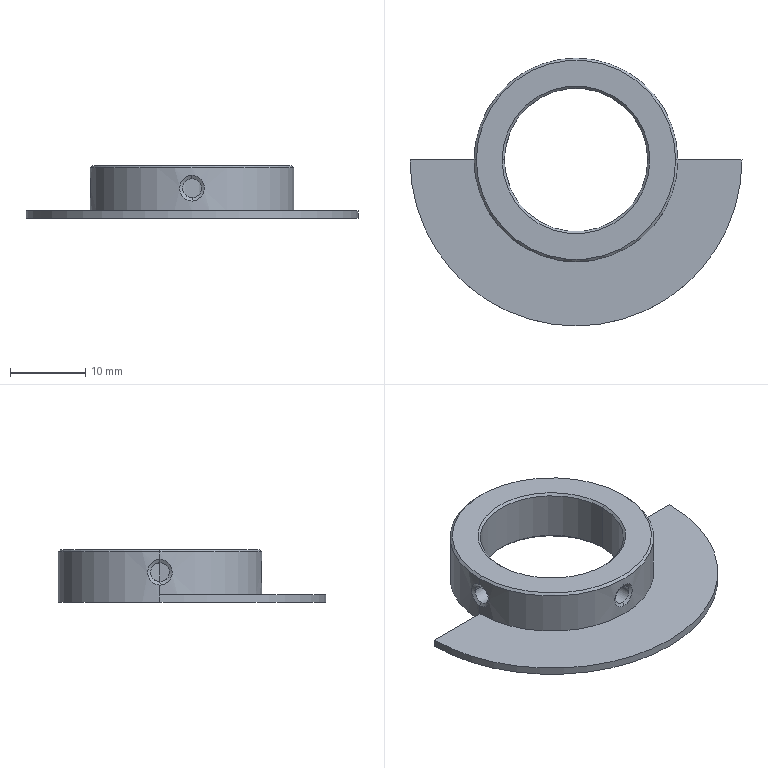Part | NX | 1 solid | 24 faces | box 44 x 35.5 x 7 mm | volume 2448 mm3 | cylinder 9 | cone 6 | plane 5 | spline 4 | commonest cylinder face diameters 2.5 x4 19 x2 27 x2 44 x1
STEP:
#1=CARTESIAN_POINT('',(13.2,0.,7.));
#2=VERTEX_POINT('',#1);
#3=CARTESIAN_POINT('',(-13.2,0.,7.));
#4=VERTEX_POINT('',#3);
#5=CARTESIAN_POINT('',(0.,0.,7.));
#6=DIRECTION('',(0.,0.,-1.));
#7=DIRECTION('',(-1.,0.,0.));
#8=AXIS2_PLACEMENT_3D('',#5,#6,#7);
#9=CIRCLE('',#8,13.2);
#10=EDGE_CURVE('',#2,#4,#9,.T.);
#11=ORIENTED_EDGE('',*,*,#10,.F.);
#12=CARTESIAN_POINT('',(0.,0.,7.));
#13=DIRECTION('',(0.,0.,-1.));
#14=DIRECTION('',(-1.,0.,0.));
#15=AXIS2_PLACEMENT_3D('',#12,#13,#14);
#16=CIRCLE('',#15,13.2);
#17=EDGE_CURVE('',#4,#2,#16,.T.);
#18=ORIENTED_EDGE('',*,*,#17,.F.);
#19=EDGE_LOOP('',(#11,#18));
#20=FACE_BOUND('',#19,.T.);
#21=CARTESIAN_POINT('',(-9.8,0.,7.));
#22=VERTEX_POINT('',#21);
#23=CARTESIAN_POINT('',(9.8,0.,7.));
#24=VERTEX_POINT('',#23);
#25=CARTESIAN_POINT('',(0.,0.,7.));
#26=DIRECTION('',(0.,0.,1.));
#27=DIRECTION('',(1.,0.,0.));
#28=AXIS2_PLACEMENT_3D('',#25,#26,#27);
#29=CIRCLE('',#28,9.8);
#30=EDGE_CURVE('',#22,#24,#29,.T.);
#31=ORIENTED_EDGE('',*,*,#30,.F.);
#32=CARTESIAN_POINT('',(0.,0.,7.));
#33=DIRECTION('',(0.,0.,1.));
#34=DIRECTION('',(1.,0.,0.));
#35=AXIS2_PLACEMENT_3D('',#32,#33,#34);
#36=CIRCLE('',#35,9.8);
#37=EDGE_CURVE('',#24,#22,#36,.T.);
#38=ORIENTED_EDGE('',*,*,#37,.F.);
#39=EDGE_LOOP('',(#31,#38));
#40=FACE_BOUND('',#39,.T.);
#41=CARTESIAN_POINT('',(0.,0.,7.));
#42=DIRECTION('',(0.,0.,1.));
#43=DIRECTION('',(1.,0.,0.));
#44=AXIS2_PLACEMENT_3D('',#41,#42,#43);
#45=PLANE('',#44);
#46=ADVANCED_FACE('',(#20,#40),#45,.T.);
#47=CARTESIAN_POINT('',(13.5,0.,0.));
#48=VERTEX_POINT('',#47);
#49=CARTESIAN_POINT('',(13.5,0.,1.));
#50=VERTEX_POINT('',#49);
#51=CARTESIAN_POINT('',(13.5,0.,0.));
#52=DIRECTION('',(0.,0.,1.));
#53=VECTOR('',#52,1000.);
#54=LINE('',#51,#53);
#55=EDGE_CURVE('',#48,#50,#54,.T.);
#56=ORIENTED_EDGE('',*,*,#55,.F.);
#57=CARTESIAN_POINT('',(-13.5,0.,0.));
#58=VERTEX_POINT('',#57);
#59=CARTESIAN_POINT('',(0.,0.,0.));
#60=DIRECTION('',(0.,0.,1.));
#61=DIRECTION('',(1.,0.,0.));
#62=AXIS2_PLACEMENT_3D('',#59,#60,#61);
#63=CIRCLE('',#62,13.5);
#64=EDGE_CURVE('',#48,#58,#63,.T.);
#65=ORIENTED_EDGE('',*,*,#64,.T.);
#66=CARTESIAN_POINT('',(-13.5,0.,1.));
#67=VERTEX_POINT('',#66);
#68=CARTESIAN_POINT('',(-13.5,0.,0.));
#69=DIRECTION('',(0.,0.,1.));
#70=VECTOR('',#69,1000.);
#71=LINE('',#68,#70);
#72=EDGE_CURVE('',#58,#67,#71,.T.);
#73=ORIENTED_EDGE('',*,*,#72,.T.);
#74=CARTESIAN_POINT('',(-13.5,0.,2.3));
#75=VERTEX_POINT('',#74);
#76=CARTESIAN_POINT('',(-13.5,0.,0.));
#77=DIRECTION('',(0.,0.,1.));
#78=VECTOR('',#77,1000.);
#79=LINE('',#76,#78);
#80=EDGE_CURVE('',#75,#67,#79,.F.);
#81=ORIENTED_EDGE('',*,*,#80,.F.);
#82=CARTESIAN_POINT('',(-13.5,0.01096,5.7));
#83=VERTEX_POINT('',#82);
#84=CARTESIAN_POINT('',(-13.5,0.,2.3));
#85=CARTESIAN_POINT('',(-13.5,0.4417,2.3));
#86=CARTESIAN_POINT('',(-13.448,1.306,2.707));
#87=CARTESIAN_POINT('',(-13.378,1.79,3.996));
#88=CARTESIAN_POINT('',(-13.447,1.313,5.283));
#89=CARTESIAN_POINT('',(-13.5,0.4559,5.697));
#90=CARTESIAN_POINT('',(-13.5,0.01096,5.7));
#91=B_SPLINE_CURVE_WITH_KNOTS('',3,(#84,#85,#86,#87,#88,#89,#90),.UNSPECIFIED.,.F.,.F.,(4,1,1,1,4),(0.,0.25,0.5,0.75,1.),.UNSPECIFIED.);
#92=EDGE_CURVE('',#83,#75,#91,.F.);
#93=ORIENTED_EDGE('',*,*,#92,.F.);
#94=CARTESIAN_POINT('',(-13.5,0.,5.7));
#95=VERTEX_POINT('',#94);
#96=CARTESIAN_POINT('',(-13.5,0.01096,5.7));
#97=CARTESIAN_POINT('',(-13.5,0.007306,5.7));
#98=CARTESIAN_POINT('',(-13.5,0.003653,5.7));
#99=CARTESIAN_POINT('',(-13.5,0.,5.7));
#100=B_SPLINE_CURVE_WITH_KNOTS('',3,(#96,#97,#98,#99),.UNSPECIFIED.,.F.,.F.,(4,4),(0.,1.),.UNSPECIFIED.);
#101=EDGE_CURVE('',#95,#83,#100,.F.);
#102=ORIENTED_EDGE('',*,*,#101,.F.);
#103=CARTESIAN_POINT('',(-13.5,0.,6.7));
#104=VERTEX_POINT('',#103);
#105=CARTESIAN_POINT('',(-13.5,0.,0.));
#106=DIRECTION('',(0.,0.,1.));
#107=VECTOR('',#106,1000.);
#108=LINE('',#105,#107);
#109=EDGE_CURVE('',#95,#104,#108,.T.);
#110=ORIENTED_EDGE('',*,*,#109,.T.);
#111=CARTESIAN_POINT('',(13.5,0.,6.7));
#112=VERTEX_POINT('',#111);
#113=CARTESIAN_POINT('',(0.,0.,6.7));
#114=DIRECTION('',(0.,0.,-1.));
#115=DIRECTION('',(-1.,0.,0.));
#116=AXIS2_PLACEMENT_3D('',#113,#114,#115);
#117=CIRCLE('',#116,13.5);
#118=EDGE_CURVE('',#104,#112,#117,.T.);
#119=ORIENTED_EDGE('',*,*,#118,.T.);
#120=CARTESIAN_POINT('',(13.5,0.,0.));
#121=DIRECTION('',(0.,0.,1.));
#122=VECTOR('',#121,1000.);
#123=LINE('',#120,#122);
#124=EDGE_CURVE('',#112,#50,#123,.F.);
#125=ORIENTED_EDGE('',*,*,#124,.T.);
#126=EDGE_LOOP('',(#56,#65,#73,#81,#93,#102,#110,#119,#125));
#127=FACE_BOUND('',#126,.T.);
#128=CARTESIAN_POINT('',(0.,0.,0.));
#129=DIRECTION('',(0.,0.,1.));
#130=DIRECTION('',(1.,0.,0.));
#131=AXIS2_PLACEMENT_3D('',#128,#129,#130);
#132=CYLINDRICAL_SURFACE('',#131,13.5);
#133=ADVANCED_FACE('',(#127),#132,.T.);
#134=CARTESIAN_POINT('',(0.009148,-13.24,2.75));
#135=VERTEX_POINT('',#134);
#136=CARTESIAN_POINT('',(1.25,-13.182,4.));
#137=VERTEX_POINT('',#136);
#138=CARTESIAN_POINT('',(0.009147,-13.24,2.75));
#139=CARTESIAN_POINT('',(0.1245,-13.24,2.751));
#140=CARTESIAN_POINT('',(0.3981,-13.236,2.779));
#141=CARTESIAN_POINT('',(0.915,-13.211,3.074));
#142=CARTESIAN_POINT('',(1.221,-13.186,3.596));
#143=CARTESIAN_POINT('',(1.25,-13.182,3.879));
#144=CARTESIAN_POINT('',(1.25,-13.182,4.));
#145=B_SPLINE_CURVE_WITH_KNOTS('',3,(#138,#139,#140,#141,#142,#143,#144),.UNSPECIFIED.,.F.,.F.,(4,1,1,1,4),(0.,0.25,0.5,0.75,1.),.UNSPECIFIED.);
#146=EDGE_CURVE('',#135,#137,#145,.T.);
#147=ORIENTED_EDGE('',*,*,#146,.F.);
#148=CARTESIAN_POINT('',(0.01305,-13.5,2.3));
#149=VERTEX_POINT('',#148);
#150=CARTESIAN_POINT('',(0.009148,-13.24,2.75));
#151=CARTESIAN_POINT('',(0.01305,-13.5,2.3));
#152=B_SPLINE_CURVE_WITH_KNOTS('',1,(#150,#151),.UNSPECIFIED.,.F.,.F.,(2,2),(0.,1.),.UNSPECIFIED.);
#153=EDGE_CURVE('',#135,#149,#152,.T.);
#154=ORIENTED_EDGE('',*,*,#153,.T.);
#155=CARTESIAN_POINT('',(-0.01314,-13.5,5.7));
#156=VERTEX_POINT('',#155);
#157=CARTESIAN_POINT('',(-0.01314,-13.5,5.7));
#158=CARTESIAN_POINT('',(0.4307,-13.5,5.704));
#159=CARTESIAN_POINT('',(1.299,-13.448,5.302));
#160=CARTESIAN_POINT('',(1.79,-13.378,4.012));
#161=CARTESIAN_POINT('',(1.317,-13.446,2.721));
#162=CARTESIAN_POINT('',(0.4589,-13.5,2.304));
#163=CARTESIAN_POINT('',(0.01305,-13.5,2.3));
#164=B_SPLINE_CURVE_WITH_KNOTS('',3,(#157,#158,#159,#160,#161,#162,#163),.UNSPECIFIED.,.F.,.F.,(4,1,1,1,4),(0.,0.25,0.5,0.75,1.),.UNSPECIFIED.);
#165=EDGE_CURVE('',#149,#156,#164,.F.);
#166=ORIENTED_EDGE('',*,*,#165,.T.);
#167=CARTESIAN_POINT('',(-0.009525,-13.24,5.25));
#168=VERTEX_POINT('',#167);
#169=CARTESIAN_POINT('',(-0.009525,-13.24,5.25));
#170=CARTESIAN_POINT('',(-0.01314,-13.5,5.7));
#171=B_SPLINE_CURVE_WITH_KNOTS('',1,(#169,#170),.UNSPECIFIED.,.F.,.F.,(2,2),(0.,1.),.UNSPECIFIED.);
#172=EDGE_CURVE('',#168,#156,#171,.T.);
#173=ORIENTED_EDGE('',*,*,#172,.F.);
#174=CARTESIAN_POINT('',(1.25,-13.182,4.));
#175=CARTESIAN_POINT('',(1.25,-13.182,4.155));
#176=CARTESIAN_POINT('',(1.178,-13.189,4.454));
#177=CARTESIAN_POINT('',(1.072,-13.198,4.655));
#178=CARTESIAN_POINT('',(0.8831,-13.212,4.907));
#179=CARTESIAN_POINT('',(0.6317,-13.225,5.086));
#180=CARTESIAN_POINT('',(0.4282,-13.234,5.187));
#181=CARTESIAN_POINT('',(0.1421,-13.24,5.251));
#182=CARTESIAN_POINT('',(-0.009525,-13.24,5.25));
#183=B_SPLINE_CURVE_WITH_KNOTS('',3,(#174,#175,#176,#177,#178,#179,#180,#181,#182),.UNSPECIFIED.,.F.,.F.,(4,1,1,1,1,1,4),(0.,0.25,0.375,0.5,0.625,0.75,1.),.UNSPECIFIED.);
#184=EDGE_CURVE('',#137,#168,#183,.T.);
#185=ORIENTED_EDGE('',*,*,#184,.F.);
#186=EDGE_LOOP('',(#147,#154,#166,#173,#185));
#187=FACE_BOUND('',#186,.T.);
#188=CARTESIAN_POINT('',(0.009148,-13.24,2.75));
#189=CARTESIAN_POINT('',(0.01305,-13.5,2.3));
#190=CARTESIAN_POINT('',(0.07196,-13.24,2.75));
#191=CARTESIAN_POINT('',(0.09975,-13.5,2.301));
#192=CARTESIAN_POINT('',(0.1349,-13.24,2.756));
#193=CARTESIAN_POINT('',(0.1865,-13.499,2.309));
#194=CARTESIAN_POINT('',(0.3998,-13.236,2.798));
#195=CARTESIAN_POINT('',(0.5485,-13.492,2.373));
#196=CARTESIAN_POINT('',(0.5907,-13.228,2.879));
#197=CARTESIAN_POINT('',(0.8061,-13.478,2.497));
#198=CARTESIAN_POINT('',(0.9215,-13.209,3.13));
#199=CARTESIAN_POINT('',(1.233,-13.445,2.855));
#200=CARTESIAN_POINT('',(1.055,-13.199,3.297));
#201=CARTESIAN_POINT('',(1.396,-13.428,3.083));
#202=CARTESIAN_POINT('',(1.227,-13.185,3.681));
#203=CARTESIAN_POINT('',(1.603,-13.405,3.591));
#204=CARTESIAN_POINT('',(1.263,-13.181,3.894));
#205=CARTESIAN_POINT('',(1.645,-13.399,3.862));
#206=CARTESIAN_POINT('',(1.228,-13.184,4.314));
#207=CARTESIAN_POINT('',(1.604,-13.404,4.406));
#208=CARTESIAN_POINT('',(1.157,-13.191,4.518));
#209=CARTESIAN_POINT('',(1.521,-13.415,4.669));
#210=CARTESIAN_POINT('',(0.925,-13.209,4.866));
#211=CARTESIAN_POINT('',(1.235,-13.444,5.14));
#212=CARTESIAN_POINT('',(0.7682,-13.219,5.007));
#213=CARTESIAN_POINT('',(1.037,-13.462,5.34));
#214=CARTESIAN_POINT('',(0.4042,-13.235,5.201));
#215=CARTESIAN_POINT('',(0.5571,-13.491,5.622));
#216=CARTESIAN_POINT('',(0.2041,-13.24,5.25));
#217=CARTESIAN_POINT('',(0.2808,-13.5,5.7));
#218=CARTESIAN_POINT('',(-0.003196,-13.24,5.25));
#219=CARTESIAN_POINT('',(-0.004398,-13.5,5.7));
#220=CARTESIAN_POINT('',(-0.006359,-13.24,5.25));
#221=CARTESIAN_POINT('',(-0.008773,-13.5,5.7));
#222=CARTESIAN_POINT('',(-0.009525,-13.24,5.25));
#223=CARTESIAN_POINT('',(-0.01314,-13.5,5.7));
#224=B_SPLINE_SURFACE_WITH_KNOTS('',3,1,((#188,#189),(#190,#191),(#192,#193),(#194,#195),(#196,#197),(#198,#199),(#200,#201),(#202,#203),(#204,#205),(#206,#207),(#208,#209),(#210,#211),(#212,#213),(#214,#215),(#216,#217),(#218,#219),(#220,#221),(#222,#223)),.RULED_SURF.,.F.,.F.,.F.,(4,2,2,2,2,2,2,2,4),(2,2),(4.613,4.839,5.568,6.302,7.029,7.759,8.489,9.216,9.227),(0.,1.),.UNSPECIFIED.);
#225=ADVANCED_FACE('',(#187),#224,.F.);
#226=CARTESIAN_POINT('',(0.,0.,1.));
#227=DIRECTION('',(0.,0.,1.));
#228=DIRECTION('',(1.,0.,0.));
#229=AXIS2_PLACEMENT_3D('',#226,#227,#228);
#230=CIRCLE('',#229,13.5);
#231=EDGE_CURVE('',#67,#50,#230,.T.);
#232=ORIENTED_EDGE('',*,*,#231,.F.);
#233=CARTESIAN_POINT('',(-22.,0.,1.));
#234=VERTEX_POINT('',#233);
#235=CARTESIAN_POINT('',(-22.,0.,1.));
#236=DIRECTION('',(1.,0.,0.));
#237=VECTOR('',#236,1000.);
#238=LINE('',#235,#237);
#239=EDGE_CURVE('',#234,#67,#238,.T.);
#240=ORIENTED_EDGE('',*,*,#239,.F.);
#241=CARTESIAN_POINT('',(22.,0.,1.));
#242=VERTEX_POINT('',#241);
#243=CARTESIAN_POINT('',(0.,0.,1.));
#244=DIRECTION('',(0.,0.,-1.));
#245=DIRECTION('',(1.,0.,0.));
#246=AXIS2_PLACEMENT_3D('',#243,#244,#245);
#247=CIRCLE('',#246,22.);
#248=EDGE_CURVE('',#242,#234,#247,.T.);
#249=ORIENTED_EDGE('',*,*,#248,.F.);
#250=CARTESIAN_POINT('',(13.5,0.,1.));
#251=DIRECTION('',(1.,0.,0.));
#252=VECTOR('',#251,1000.);
#253=LINE('',#250,#252);
#254=EDGE_CURVE('',#50,#242,#253,.T.);
#255=ORIENTED_EDGE('',*,*,#254,.F.);
#256=EDGE_LOOP('',(#232,#240,#249,#255));
#257=FACE_BOUND('',#256,.T.);
#258=CARTESIAN_POINT('',(0.,0.,1.));
#259=DIRECTION('',(0.,0.,1.));
#260=DIRECTION('',(1.,0.,0.));
#261=AXIS2_PLACEMENT_3D('',#258,#259,#260);
#262=PLANE('',#261);
#263=ADVANCED_FACE('',(#257),#262,.T.);
#264=ORIENTED_EDGE('',*,*,#55,.T.);
#265=ORIENTED_EDGE('',*,*,#254,.T.);
#266=CARTESIAN_POINT('',(22.,0.,0.));
#267=VERTEX_POINT('',#266);
#268=CARTESIAN_POINT('',(22.,0.,0.));
#269=DIRECTION('',(0.,0.,1.));
#270=VECTOR('',#269,1000.);
#271=LINE('',#268,#270);
#272=EDGE_CURVE('',#267,#242,#271,.T.);
#273=ORIENTED_EDGE('',*,*,#272,.F.);
#274=CARTESIAN_POINT('',(13.5,0.,0.));
#275=DIRECTION('',(1.,0.,0.));
#276=VECTOR('',#275,1000.);
#277=LINE('',#274,#276);
#278=EDGE_CURVE('',#48,#267,#277,.T.);
#279=ORIENTED_EDGE('',*,*,#278,.F.);
#280=EDGE_LOOP('',(#264,#265,#273,#279));
#281=FACE_BOUND('',#280,.T.);
#282=CARTESIAN_POINT('',(22.,0.,0.));
#283=DIRECTION('',(0.,1.,0.));
#284=DIRECTION('',(1.,0.,0.));
#285=AXIS2_PLACEMENT_3D('',#282,#283,#284);
#286=PLANE('',#285);
#287=ADVANCED_FACE('',(#281),#286,.T.);
#288=ORIENTED_EDGE('',*,*,#64,.F.);
#289=ORIENTED_EDGE('',*,*,#278,.T.);
#290=CARTESIAN_POINT('',(-22.,0.,0.));
#291=VERTEX_POINT('',#290);
#292=CARTESIAN_POINT('',(0.,0.,0.));
#293=DIRECTION('',(0.,0.,1.));
#294=DIRECTION('',(-1.,0.,0.));
#295=AXIS2_PLACEMENT_3D('',#292,#293,#294);
#296=CIRCLE('',#295,22.);
#297=EDGE_CURVE('',#291,#267,#296,.T.);
#298=ORIENTED_EDGE('',*,*,#297,.F.);
#299=CARTESIAN_POINT('',(-22.,0.,0.));
#300=DIRECTION('',(1.,0.,0.));
#301=VECTOR('',#300,1000.);
#302=LINE('',#299,#301);
#303=EDGE_CURVE('',#291,#58,#302,.T.);
#304=ORIENTED_EDGE('',*,*,#303,.T.);
#305=EDGE_LOOP('',(#288,#289,#298,#304));
#306=FACE_BOUND('',#305,.T.);
#307=CARTESIAN_POINT('',(-9.8,0.,0.));
#308=VERTEX_POINT('',#307);
#309=CARTESIAN_POINT('',(9.8,0.,0.));
#310=VERTEX_POINT('',#309);
#311=CARTESIAN_POINT('',(0.,0.,0.));
#312=DIRECTION('',(0.,0.,-1.));
#313=DIRECTION('',(-1.,0.,0.));
#314=AXIS2_PLACEMENT_3D('',#311,#312,#313);
#315=CIRCLE('',#314,9.8);
#316=EDGE_CURVE('',#308,#310,#315,.T.);
#317=ORIENTED_EDGE('',*,*,#316,.F.);
#318=CARTESIAN_POINT('',(0.,0.,0.));
#319=DIRECTION('',(0.,0.,-1.));
#320=DIRECTION('',(-1.,0.,0.));
#321=AXIS2_PLACEMENT_3D('',#318,#319,#320);
#322=CIRCLE('',#321,9.8);
#323=EDGE_CURVE('',#310,#308,#322,.T.);
#324=ORIENTED_EDGE('',*,*,#323,.F.);
#325=EDGE_LOOP('',(#317,#324));
#326=FACE_BOUND('',#325,.T.);
#327=CARTESIAN_POINT('',(0.,0.,0.));
#328=DIRECTION('',(0.,0.,1.));
#329=DIRECTION('',(1.,0.,0.));
#330=AXIS2_PLACEMENT_3D('',#327,#328,#329);
#331=PLANE('',#330);
#332=ADVANCED_FACE('',(#306,#326),#331,.F.);
#333=CARTESIAN_POINT('',(9.5,0.,0.3));
#334=VERTEX_POINT('',#333);
#335=CARTESIAN_POINT('',(-9.5,0.,0.3));
#336=VERTEX_POINT('',#335);
#337=CARTESIAN_POINT('',(0.,0.,0.3));
#338=DIRECTION('',(0.,0.,-1.));
#339=DIRECTION('',(-1.,0.,0.));
#340=AXIS2_PLACEMENT_3D('',#337,#338,#339);
#341=CIRCLE('',#340,9.5);
#342=EDGE_CURVE('',#334,#336,#341,.T.);
#343=ORIENTED_EDGE('',*,*,#342,.T.);
#344=CARTESIAN_POINT('',(-9.5,0.,2.75));
#345=VERTEX_POINT('',#344);
#346=CARTESIAN_POINT('',(-9.5,0.,0.));
#347=DIRECTION('',(0.,0.,1.));
#348=VECTOR('',#347,1000.);
#349=LINE('',#346,#348);
#350=EDGE_CURVE('',#336,#345,#349,.T.);
#351=ORIENTED_EDGE('',*,*,#350,.T.);
#352=CARTESIAN_POINT('',(-9.417,-1.25,4.));
#353=VERTEX_POINT('',#352);
#354=CARTESIAN_POINT('',(-9.5,0.,2.75));
#355=CARTESIAN_POINT('',(-9.5,-0.6631,2.75));
#356=CARTESIAN_POINT('',(-9.417,-1.249,3.335));
#357=CARTESIAN_POINT('',(-9.417,-1.25,4.));
#358=B_SPLINE_CURVE_WITH_KNOTS('',3,(#354,#355,#356,#357),.UNSPECIFIED.,.F.,.F.,(4,4),(0.,1.),.UNSPECIFIED.);
#359=EDGE_CURVE('',#345,#353,#358,.T.);
#360=ORIENTED_EDGE('',*,*,#359,.T.);
#361=CARTESIAN_POINT('',(-9.5,0.,5.25));
#362=VERTEX_POINT('',#361);
#363=CARTESIAN_POINT('',(-9.417,-1.25,4.));
#364=CARTESIAN_POINT('',(-9.417,-1.249,4.664));
#365=CARTESIAN_POINT('',(-9.5,-0.6634,5.25));
#366=CARTESIAN_POINT('',(-9.5,0.,5.25));
#367=B_SPLINE_CURVE_WITH_KNOTS('',3,(#363,#364,#365,#366),.UNSPECIFIED.,.F.,.F.,(4,4),(0.,1.),.UNSPECIFIED.);
#368=EDGE_CURVE('',#353,#362,#367,.T.);
#369=ORIENTED_EDGE('',*,*,#368,.T.);
#370=CARTESIAN_POINT('',(-9.5,0.,6.7));
#371=VERTEX_POINT('',#370);
#372=CARTESIAN_POINT('',(-9.5,0.,0.));
#373=DIRECTION('',(0.,0.,1.));
#374=VECTOR('',#373,1000.);
#375=LINE('',#372,#374);
#376=EDGE_CURVE('',#371,#362,#375,.F.);
#377=ORIENTED_EDGE('',*,*,#376,.F.);
#378=CARTESIAN_POINT('',(9.5,0.,6.7));
#379=VERTEX_POINT('',#378);
#380=CARTESIAN_POINT('',(0.,0.,6.7));
#381=DIRECTION('',(0.,0.,1.));
#382=DIRECTION('',(1.,0.,0.));
#383=AXIS2_PLACEMENT_3D('',#380,#381,#382);
#384=CIRCLE('',#383,9.5);
#385=EDGE_CURVE('',#371,#379,#384,.T.);
#386=ORIENTED_EDGE('',*,*,#385,.T.);
#387=CARTESIAN_POINT('',(9.5,0.,0.));
#388=DIRECTION('',(0.,0.,1.));
#389=VECTOR('',#388,1000.);
#390=LINE('',#387,#389);
#391=EDGE_CURVE('',#379,#334,#390,.F.);
#392=ORIENTED_EDGE('',*,*,#391,.T.);
#393=EDGE_LOOP('',(#343,#351,#360,#369,#377,#386,#392));
#394=FACE_BOUND('',#393,.T.);
#395=CARTESIAN_POINT('',(1.25,-9.417,4.));
#396=VERTEX_POINT('',#395);
#397=CARTESIAN_POINT('',(-1.25,-9.417,4.));
#398=VERTEX_POINT('',#397);
#399=CARTESIAN_POINT('',(-1.25,-9.417,4.));
#400=CARTESIAN_POINT('',(-1.25,-9.417,3.668));
#401=CARTESIAN_POINT('',(-0.9802,-9.459,3.024));
#402=CARTESIAN_POINT('',(0.0002555,-9.521,2.613));
#403=CARTESIAN_POINT('',(0.9792,-9.459,3.023));
#404=CARTESIAN_POINT('',(1.25,-9.417,3.668));
#405=CARTESIAN_POINT('',(1.25,-9.417,4.));
#406=B_SPLINE_CURVE_WITH_KNOTS('',3,(#399,#400,#401,#402,#403,#404,#405),.UNSPECIFIED.,.F.,.F.,(4,1,1,1,4),(0.,0.25,0.5,0.75,1.),.UNSPECIFIED.);
#407=EDGE_CURVE('',#396,#398,#406,.F.);
#408=ORIENTED_EDGE('',*,*,#407,.F.);
#409=CARTESIAN_POINT('',(1.25,-9.417,4.));
#410=CARTESIAN_POINT('',(1.25,-9.417,4.332));
#411=CARTESIAN_POINT('',(0.9799,-9.459,4.976));
#412=CARTESIAN_POINT('',(0.00004699,-9.521,5.387));
#413=CARTESIAN_POINT('',(-0.9802,-9.459,4.976));
#414=CARTESIAN_POINT('',(-1.25,-9.417,4.332));
#415=CARTESIAN_POINT('',(-1.25,-9.417,4.));
#416=B_SPLINE_CURVE_WITH_KNOTS('',3,(#409,#410,#411,#412,#413,#414,#415),.UNSPECIFIED.,.F.,.F.,(4,1,1,1,4),(0.,0.25,0.5,0.75,1.),.UNSPECIFIED.);
#417=EDGE_CURVE('',#398,#396,#416,.F.);
#418=ORIENTED_EDGE('',*,*,#417,.F.);
#419=EDGE_LOOP('',(#408,#418));
#420=FACE_BOUND('',#419,.T.);
#421=CARTESIAN_POINT('',(0.,0.,0.));
#422=DIRECTION('',(0.,0.,1.));
#423=DIRECTION('',(1.,0.,0.));
#424=AXIS2_PLACEMENT_3D('',#421,#422,#423);
#425=CYLINDRICAL_SURFACE('',#424,9.5);
#426=ADVANCED_FACE('',(#394,#420),#425,.F.);
#427=ORIENTED_EDGE('',*,*,#72,.F.);
#428=ORIENTED_EDGE('',*,*,#303,.F.);
#429=CARTESIAN_POINT('',(-22.,0.,0.));
#430=DIRECTION('',(0.,0.,1.));
#431=VECTOR('',#430,1000.);
#432=LINE('',#429,#431);
#433=EDGE_CURVE('',#291,#234,#432,.T.);
#434=ORIENTED_EDGE('',*,*,#433,.T.);
#435=ORIENTED_EDGE('',*,*,#239,.T.);
#436=EDGE_LOOP('',(#427,#428,#434,#435));
#437=FACE_BOUND('',#436,.T.);
#438=CARTESIAN_POINT('',(-13.5,0.,0.));
#439=DIRECTION('',(0.,1.,0.));
#440=DIRECTION('',(1.,0.,0.));
#441=AXIS2_PLACEMENT_3D('',#438,#439,#440);
#442=PLANE('',#441);
#443=ADVANCED_FACE('',(#437),#442,.T.);
#444=ORIENTED_EDGE('',*,*,#297,.T.);
#445=ORIENTED_EDGE('',*,*,#272,.T.);
#446=ORIENTED_EDGE('',*,*,#248,.T.);
#447=ORIENTED_EDGE('',*,*,#433,.F.);
#448=EDGE_LOOP('',(#444,#445,#446,#447));
#449=FACE_BOUND('',#448,.T.);
#450=CARTESIAN_POINT('',(0.,0.,0.));
#451=DIRECTION('',(0.,0.,1.));
#452=DIRECTION('',(1.,0.,0.));
#453=AXIS2_PLACEMENT_3D('',#450,#451,#452);
#454=CYLINDRICAL_SURFACE('',#453,22.);
#455=ADVANCED_FACE('',(#449),#454,.T.);
#456=ORIENTED_EDGE('',*,*,#407,.T.);
#457=CARTESIAN_POINT('',(-1.25,-13.182,4.));
#458=VERTEX_POINT('',#457);
#459=CARTESIAN_POINT('',(-1.25,-13.5,4.));
#460=DIRECTION('',(0.,-1.,0.));
#461=VECTOR('',#460,1000.);
#462=LINE('',#459,#461);
#463=EDGE_CURVE('',#458,#398,#462,.F.);
#464=ORIENTED_EDGE('',*,*,#463,.F.);
#465=CARTESIAN_POINT('',(-1.25,-13.182,4.));
#466=CARTESIAN_POINT('',(-1.25,-13.182,3.841));
#467=CARTESIAN_POINT('',(-1.178,-13.189,3.547));
#468=CARTESIAN_POINT('',(-1.072,-13.198,3.344));
#469=CARTESIAN_POINT('',(-0.8826,-13.212,3.093));
#470=CARTESIAN_POINT('',(-0.6331,-13.225,2.915));
#471=CARTESIAN_POINT('',(-0.4278,-13.234,2.813));
#472=CARTESIAN_POINT('',(-0.1458,-13.24,2.749));
#473=CARTESIAN_POINT('',(0.009147,-13.24,2.75));
#474=B_SPLINE_CURVE_WITH_KNOTS('',3,(#465,#466,#467,#468,#469,#470,#471,#472,#473),.UNSPECIFIED.,.F.,.F.,(4,1,1,1,1,1,4),(0.,0.25,0.375,0.5,0.625,0.75,1.),.UNSPECIFIED.);
#475=EDGE_CURVE('',#458,#135,#474,.T.);
#476=ORIENTED_EDGE('',*,*,#475,.T.);
#477=ORIENTED_EDGE('',*,*,#146,.T.);
#478=CARTESIAN_POINT('',(1.25,-13.5,4.));
#479=DIRECTION('',(0.,-1.,0.));
#480=VECTOR('',#479,1000.);
#481=LINE('',#478,#480);
#482=EDGE_CURVE('',#137,#396,#481,.F.);
#483=ORIENTED_EDGE('',*,*,#482,.T.);
#484=EDGE_LOOP('',(#456,#464,#476,#477,#483));
#485=FACE_BOUND('',#484,.T.);
#486=CARTESIAN_POINT('',(0.,-13.5,4.));
#487=DIRECTION('',(0.,-1.,0.));
#488=DIRECTION('',(-1.,0.,0.));
#489=AXIS2_PLACEMENT_3D('',#486,#487,#488);
#490=CYLINDRICAL_SURFACE('',#489,1.25);
#491=ADVANCED_FACE('',(#485),#490,.F.);
#492=ORIENTED_EDGE('',*,*,#368,.F.);
#493=CARTESIAN_POINT('',(-13.182,-1.25,4.));
#494=VERTEX_POINT('',#493);
#495=CARTESIAN_POINT('',(-13.5,-1.25,4.));
#496=DIRECTION('',(-1.,0.,0.));
#497=VECTOR('',#496,1000.);
#498=LINE('',#495,#497);
#499=EDGE_CURVE('',#353,#494,#498,.T.);
#500=ORIENTED_EDGE('',*,*,#499,.T.);
#501=CARTESIAN_POINT('',(-13.24,0.007631,5.25));
#502=VERTEX_POINT('',#501);
#503=CARTESIAN_POINT('',(-13.182,-1.25,4.));
#504=CARTESIAN_POINT('',(-13.182,-1.25,4.159));
#505=CARTESIAN_POINT('',(-13.189,-1.179,4.452));
#506=CARTESIAN_POINT('',(-13.198,-1.072,4.656));
#507=CARTESIAN_POINT('',(-13.212,-0.8832,4.907));
#508=CARTESIAN_POINT('',(-13.225,-0.6338,5.085));
#509=CARTESIAN_POINT('',(-13.234,-0.429,5.187));
#510=CARTESIAN_POINT('',(-13.24,-0.1471,5.251));
#511=CARTESIAN_POINT('',(-13.24,0.00763,5.25));
#512=B_SPLINE_CURVE_WITH_KNOTS('',3,(#503,#504,#505,#506,#507,#508,#509,#510,#511),.UNSPECIFIED.,.F.,.F.,(4,1,1,1,1,1,4),(0.,0.25,0.375,0.5,0.625,0.75,1.),.UNSPECIFIED.);
#513=EDGE_CURVE('',#494,#502,#512,.T.);
#514=ORIENTED_EDGE('',*,*,#513,.T.);
#515=CARTESIAN_POINT('',(-13.182,1.25,4.));
#516=VERTEX_POINT('',#515);
#517=CARTESIAN_POINT('',(-13.24,0.00763,5.25));
#518=CARTESIAN_POINT('',(-13.24,0.1583,5.249));
#519=CARTESIAN_POINT('',(-13.234,0.4417,5.182));
#520=CARTESIAN_POINT('',(-13.225,0.6422,5.08));
#521=CARTESIAN_POINT('',(-13.211,0.8894,4.9));
#522=CARTESIAN_POINT('',(-13.197,1.076,4.649));
#523=CARTESIAN_POINT('',(-13.188,1.179,4.449));
#524=CARTESIAN_POINT('',(-13.182,1.25,4.158));
#525=CARTESIAN_POINT('',(-13.182,1.25,4.));
#526=B_SPLINE_CURVE_WITH_KNOTS('',3,(#517,#518,#519,#520,#521,#522,#523,#524,#525),.UNSPECIFIED.,.F.,.F.,(4,1,1,1,1,1,4),(0.,0.25,0.375,0.5,0.625,0.75,1.),.UNSPECIFIED.);
#527=EDGE_CURVE('',#502,#516,#526,.T.);
#528=ORIENTED_EDGE('',*,*,#527,.T.);
#529=CARTESIAN_POINT('',(-9.417,1.25,4.));
#530=VERTEX_POINT('',#529);
#531=CARTESIAN_POINT('',(-13.5,1.25,4.));
#532=DIRECTION('',(-1.,0.,0.));
#533=VECTOR('',#532,1000.);
#534=LINE('',#531,#533);
#535=EDGE_CURVE('',#530,#516,#534,.T.);
#536=ORIENTED_EDGE('',*,*,#535,.F.);
#537=CARTESIAN_POINT('',(-9.417,1.25,4.));
#538=CARTESIAN_POINT('',(-9.417,1.25,4.155));
#539=CARTESIAN_POINT('',(-9.426,1.181,4.444));
#540=CARTESIAN_POINT('',(-9.439,1.079,4.645));
#541=CARTESIAN_POINT('',(-9.459,0.8946,4.895));
#542=CARTESIAN_POINT('',(-9.478,0.6462,5.077));
#543=CARTESIAN_POINT('',(-9.491,0.4429,5.182));
#544=CARTESIAN_POINT('',(-9.5,0.1549,5.25));
#545=CARTESIAN_POINT('',(-9.5,0.,5.25));
#546=B_SPLINE_CURVE_WITH_KNOTS('',3,(#537,#538,#539,#540,#541,#542,#543,#544,#545),.UNSPECIFIED.,.F.,.F.,(4,1,1,1,1,1,4),(0.,0.25,0.375,0.5,0.625,0.75,1.),.UNSPECIFIED.);
#547=EDGE_CURVE('',#362,#530,#546,.F.);
#548=ORIENTED_EDGE('',*,*,#547,.F.);
#549=EDGE_LOOP('',(#492,#500,#514,#528,#536,#548));
#550=FACE_BOUND('',#549,.T.);
#551=CARTESIAN_POINT('',(-13.5,0.,4.));
#552=DIRECTION('',(-1.,0.,0.));
#553=DIRECTION('',(0.,1.,0.));
#554=AXIS2_PLACEMENT_3D('',#551,#552,#553);
#555=CYLINDRICAL_SURFACE('',#554,1.25);
#556=ADVANCED_FACE('',(#550),#555,.F.);
#557=ORIENTED_EDGE('',*,*,#513,.F.);
#558=CARTESIAN_POINT('',(-13.24,-0.008007,2.75));
#559=VERTEX_POINT('',#558);
#560=CARTESIAN_POINT('',(-13.24,-0.008007,2.75));
#561=CARTESIAN_POINT('',(-13.24,-0.1601,2.751));
#562=CARTESIAN_POINT('',(-13.234,-0.4439,2.819));
#563=CARTESIAN_POINT('',(-13.225,-0.6419,2.92));
#564=CARTESIAN_POINT('',(-13.211,-0.8903,3.101));
#565=CARTESIAN_POINT('',(-13.198,-1.073,3.347));
#566=CARTESIAN_POINT('',(-13.188,-1.181,3.553));
#567=CARTESIAN_POINT('',(-13.182,-1.25,3.842));
#568=CARTESIAN_POINT('',(-13.182,-1.25,4.));
#569=B_SPLINE_CURVE_WITH_KNOTS('',3,(#560,#561,#562,#563,#564,#565,#566,#567,#568),.UNSPECIFIED.,.F.,.F.,(4,1,1,1,1,1,4),(0.,0.25,0.375,0.5,0.625,0.75,1.),.UNSPECIFIED.);
#570=EDGE_CURVE('',#559,#494,#569,.T.);
#571=ORIENTED_EDGE('',*,*,#570,.F.);
#572=CARTESIAN_POINT('',(-13.5,-0.01105,2.3));
#573=VERTEX_POINT('',#572);
#574=CARTESIAN_POINT('',(-13.24,-0.008007,2.75));
#575=CARTESIAN_POINT('',(-13.5,-0.01105,2.3));
#576=B_SPLINE_CURVE_WITH_KNOTS('',1,(#574,#575),.UNSPECIFIED.,.F.,.F.,(2,2),(0.,1.),.UNSPECIFIED.);
#577=EDGE_CURVE('',#559,#573,#576,.T.);
#578=ORIENTED_EDGE('',*,*,#577,.T.);
#579=CARTESIAN_POINT('',(-13.5,0.,5.7));
#580=CARTESIAN_POINT('',(-13.5,-0.4479,5.699));
#581=CARTESIAN_POINT('',(-13.448,-1.303,5.293));
#582=CARTESIAN_POINT('',(-13.378,-1.79,4.006));
#583=CARTESIAN_POINT('',(-13.446,-1.314,2.718));
#584=CARTESIAN_POINT('',(-13.5,-0.4559,2.303));
#585=CARTESIAN_POINT('',(-13.5,-0.01105,2.3));
#586=B_SPLINE_CURVE_WITH_KNOTS('',3,(#579,#580,#581,#582,#583,#584,#585),.UNSPECIFIED.,.F.,.F.,(4,1,1,1,4),(0.,0.25,0.5,0.75,1.),.UNSPECIFIED.);
#587=EDGE_CURVE('',#573,#95,#586,.F.);
#588=ORIENTED_EDGE('',*,*,#587,.T.);
#589=ORIENTED_EDGE('',*,*,#101,.T.);
#590=CARTESIAN_POINT('',(-13.24,0.007631,5.25));
#591=CARTESIAN_POINT('',(-13.5,0.01096,5.7));
#592=B_SPLINE_CURVE_WITH_KNOTS('',1,(#590,#591),.UNSPECIFIED.,.F.,.F.,(2,2),(0.,1.),.UNSPECIFIED.);
#593=EDGE_CURVE('',#502,#83,#592,.T.);
#594=ORIENTED_EDGE('',*,*,#593,.F.);
#595=EDGE_LOOP('',(#557,#571,#578,#588,#589,#594));
#596=FACE_BOUND('',#595,.T.);
#597=CARTESIAN_POINT('',(-13.24,-0.008007,2.75));
#598=CARTESIAN_POINT('',(-13.5,-0.01105,2.3));
#599=CARTESIAN_POINT('',(-13.24,-0.01372,2.75));
#600=CARTESIAN_POINT('',(-13.5,-0.01893,2.3));
#601=CARTESIAN_POINT('',(-13.24,-0.01944,2.75));
#602=CARTESIAN_POINT('',(-13.5,-0.02682,2.3));
#603=CARTESIAN_POINT('',(-13.24,-0.04897,2.751));
#604=CARTESIAN_POINT('',(-13.5,-0.06756,2.301));
#605=CARTESIAN_POINT('',(-13.24,-0.07275,2.752));
#606=CARTESIAN_POINT('',(-13.5,-0.1004,2.303));
#607=CARTESIAN_POINT('',(-13.239,-0.1958,2.761));
#608=CARTESIAN_POINT('',(-13.498,-0.2697,2.318));
#609=CARTESIAN_POINT('',(-13.237,-0.2935,2.781));
#610=CARTESIAN_POINT('',(-13.495,-0.4045,2.348));
#611=CARTESIAN_POINT('',(-13.229,-0.5846,2.876));
#612=CARTESIAN_POINT('',(-13.479,-0.7967,2.49));
#613=CARTESIAN_POINT('',(-13.219,-0.7622,2.987));
#614=CARTESIAN_POINT('',(-13.462,-1.029,2.655));
#615=CARTESIAN_POINT('',(-13.2,-1.049,3.289));
#616=CARTESIAN_POINT('',(-13.429,-1.39,3.073));
#617=CARTESIAN_POINT('',(-13.191,-1.154,3.475));
#618=CARTESIAN_POINT('',(-13.415,-1.515,3.319));
#619=CARTESIAN_POINT('',(-13.181,-1.262,3.881));
#620=CARTESIAN_POINT('',(-13.4,-1.644,3.849));
#621=CARTESIAN_POINT('',(-13.181,-1.264,4.097));
#622=CARTESIAN_POINT('',(-13.399,-1.646,4.123));
#623=CARTESIAN_POINT('',(-13.19,-1.162,4.507));
#624=CARTESIAN_POINT('',(-13.414,-1.525,4.657));
#625=CARTESIAN_POINT('',(-13.199,-1.059,4.697));
#626=CARTESIAN_POINT('',(-13.428,-1.402,4.908));
#627=CARTESIAN_POINT('',(-13.218,-0.7742,5.003));
#628=CARTESIAN_POINT('',(-13.461,-1.045,5.332));
#629=CARTESIAN_POINT('',(-13.228,-0.598,5.117));
#630=CARTESIAN_POINT('',(-13.478,-0.8148,5.499));
#631=CARTESIAN_POINT('',(-13.238,-0.2698,5.229));
#632=CARTESIAN_POINT('',(-13.496,-0.3728,5.667));
#633=CARTESIAN_POINT('',(-13.24,-0.1314,5.251));
#634=CARTESIAN_POINT('',(-13.5,-0.181,5.701));
#635=CARTESIAN_POINT('',(-13.24,0.007631,5.25));
#636=CARTESIAN_POINT('',(-13.5,0.01096,5.7));
#637=B_SPLINE_SURFACE_WITH_KNOTS('',3,1,((#597,#598),(#599,#600),(#601,#602),(#603,#604),(#605,#606),(#607,#608),(#609,#610),(#611,#612),(#613,#614),(#615,#616),(#617,#618),(#619,#620),(#621,#622),(#623,#624),(#625,#626),(#627,#628),(#629,#630),(#631,#632),(#633,#634),(#635,#636)),.RULED_SURF.,.F.,.F.,.F.,(4,2,2,2,2,2,2,2,2,4),(2,2),(0.,0.02041,0.1054,0.4605,1.193,1.92,2.648,3.383,4.114,4.613),(0.,1.),.UNSPECIFIED.);
#638=ADVANCED_FACE('',(#596),#637,.F.);
#639=CARTESIAN_POINT('',(0.,0.,6.7));
#640=DIRECTION('',(0.,0.,-1.));
#641=DIRECTION('',(-1.,0.,0.));
#642=AXIS2_PLACEMENT_3D('',#639,#640,#641);
#643=CIRCLE('',#642,13.5);
#644=EDGE_CURVE('',#112,#104,#643,.T.);
#645=ORIENTED_EDGE('',*,*,#644,.F.);
#646=CARTESIAN_POINT('',(13.5,0.,6.7));
#647=DIRECTION('',(0.7071,0.,-0.7071));
#648=VECTOR('',#647,1000.);
#649=LINE('',#646,#648);
#650=EDGE_CURVE('',#112,#2,#649,.F.);
#651=ORIENTED_EDGE('',*,*,#650,.T.);
#652=ORIENTED_EDGE('',*,*,#10,.T.);
#653=CARTESIAN_POINT('',(-13.5,0.,6.7));
#654=DIRECTION('',(-0.7071,0.,-0.7071));
#655=VECTOR('',#654,1000.);
#656=LINE('',#653,#655);
#657=EDGE_CURVE('',#104,#4,#656,.F.);
#658=ORIENTED_EDGE('',*,*,#657,.F.);
#659=EDGE_LOOP('',(#645,#651,#652,#658));
#660=FACE_BOUND('',#659,.T.);
#661=CARTESIAN_POINT('',(0.,0.,6.7));
#662=DIRECTION('',(0.,0.,-1.));
#663=DIRECTION('',(-1.,0.,0.));
#664=AXIS2_PLACEMENT_3D('',#661,#662,#663);
#665=CONICAL_SURFACE('',#664,13.5,0.7854);
#666=ADVANCED_FACE('',(#660),#665,.T.);
#667=ORIENTED_EDGE('',*,*,#30,.T.);
#668=CARTESIAN_POINT('',(9.8,0.,7.));
#669=DIRECTION('',(0.7071,0.,0.7071));
#670=VECTOR('',#669,1000.);
#671=LINE('',#668,#670);
#672=EDGE_CURVE('',#379,#24,#671,.T.);
#673=ORIENTED_EDGE('',*,*,#672,.F.);
#674=ORIENTED_EDGE('',*,*,#385,.F.);
#675=CARTESIAN_POINT('',(-9.8,0.,7.));
#676=DIRECTION('',(-0.7071,0.,0.7071));
#677=VECTOR('',#676,1000.);
#678=LINE('',#675,#677);
#679=EDGE_CURVE('',#371,#22,#678,.T.);
#680=ORIENTED_EDGE('',*,*,#679,.T.);
#681=EDGE_LOOP('',(#667,#673,#674,#680));
#682=FACE_BOUND('',#681,.T.);
#683=CARTESIAN_POINT('',(0.,0.,7.));
#684=DIRECTION('',(0.,0.,1.));
#685=DIRECTION('',(1.,0.,0.));
#686=AXIS2_PLACEMENT_3D('',#683,#684,#685);
#687=CONICAL_SURFACE('',#686,9.8,0.7854);
#688=ADVANCED_FACE('',(#682),#687,.F.);
#689=ORIENTED_EDGE('',*,*,#342,.F.);
#690=CARTESIAN_POINT('',(9.8,0.,0.));
#691=DIRECTION('',(0.7071,0.,-0.7071));
#692=VECTOR('',#691,1000.);
#693=LINE('',#690,#692);
#694=EDGE_CURVE('',#334,#310,#693,.T.);
#695=ORIENTED_EDGE('',*,*,#694,.T.);
#696=ORIENTED_EDGE('',*,*,#323,.T.);
#697=CARTESIAN_POINT('',(-9.8,0.,0.));
#698=DIRECTION('',(-0.7071,0.,-0.7071));
#699=VECTOR('',#698,1000.);
#700=LINE('',#697,#699);
#701=EDGE_CURVE('',#336,#308,#700,.T.);
#702=ORIENTED_EDGE('',*,*,#701,.F.);
#703=EDGE_LOOP('',(#689,#695,#696,#702));
#704=FACE_BOUND('',#703,.T.);
#705=CARTESIAN_POINT('',(0.,0.,0.));
#706=DIRECTION('',(0.,0.,-1.));
#707=DIRECTION('',(-1.,0.,0.));
#708=AXIS2_PLACEMENT_3D('',#705,#706,#707);
#709=CONICAL_SURFACE('',#708,9.8,0.7854);
#710=ADVANCED_FACE('',(#704),#709,.F.);
#711=ORIENTED_EDGE('',*,*,#657,.T.);
#712=ORIENTED_EDGE('',*,*,#17,.T.);
#713=ORIENTED_EDGE('',*,*,#650,.F.);
#714=ORIENTED_EDGE('',*,*,#118,.F.);
#715=EDGE_LOOP('',(#711,#712,#713,#714));
#716=FACE_BOUND('',#715,.T.);
#717=CARTESIAN_POINT('',(0.,0.,6.7));
#718=DIRECTION('',(0.,0.,-1.));
#719=DIRECTION('',(-1.,0.,0.));
#720=AXIS2_PLACEMENT_3D('',#717,#718,#719);
#721=CONICAL_SURFACE('',#720,13.5,0.7854);
#722=ADVANCED_FACE('',(#716),#721,.T.);
#723=ORIENTED_EDGE('',*,*,#535,.T.);
#724=CARTESIAN_POINT('',(-13.182,1.25,4.));
#725=CARTESIAN_POINT('',(-13.182,1.25,3.845));
#726=CARTESIAN_POINT('',(-13.189,1.179,3.547));
#727=CARTESIAN_POINT('',(-13.198,1.072,3.345));
#728=CARTESIAN_POINT('',(-13.212,0.8837,3.094));
#729=CARTESIAN_POINT('',(-13.225,0.6324,2.914));
#730=CARTESIAN_POINT('',(-13.234,0.4295,2.813));
#731=CARTESIAN_POINT('',(-13.24,0.1435,2.749));
#732=CARTESIAN_POINT('',(-13.24,-0.008007,2.75));
#733=B_SPLINE_CURVE_WITH_KNOTS('',3,(#724,#725,#726,#727,#728,#729,#730,#731,#732),.UNSPECIFIED.,.F.,.F.,(4,1,1,1,1,1,4),(0.,0.25,0.375,0.5,0.625,0.75,1.),.UNSPECIFIED.);
#734=EDGE_CURVE('',#516,#559,#733,.T.);
#735=ORIENTED_EDGE('',*,*,#734,.T.);
#736=ORIENTED_EDGE('',*,*,#570,.T.);
#737=ORIENTED_EDGE('',*,*,#499,.F.);
#738=ORIENTED_EDGE('',*,*,#359,.F.);
#739=CARTESIAN_POINT('',(-9.5,0.,2.75));
#740=CARTESIAN_POINT('',(-9.5,0.1548,2.75));
#741=CARTESIAN_POINT('',(-9.491,0.443,2.818));
#742=CARTESIAN_POINT('',(-9.478,0.6461,2.922));
#743=CARTESIAN_POINT('',(-9.459,0.8947,3.105));
#744=CARTESIAN_POINT('',(-9.439,1.079,3.356));
#745=CARTESIAN_POINT('',(-9.426,1.181,3.556));
#746=CARTESIAN_POINT('',(-9.417,1.25,3.845));
#747=CARTESIAN_POINT('',(-9.417,1.25,4.));
#748=B_SPLINE_CURVE_WITH_KNOTS('',3,(#739,#740,#741,#742,#743,#744,#745,#746,#747),.UNSPECIFIED.,.F.,.F.,(4,1,1,1,1,1,4),(0.,0.25,0.375,0.5,0.625,0.75,1.),.UNSPECIFIED.);
#749=EDGE_CURVE('',#530,#345,#748,.F.);
#750=ORIENTED_EDGE('',*,*,#749,.F.);
#751=EDGE_LOOP('',(#723,#735,#736,#737,#738,#750));
#752=FACE_BOUND('',#751,.T.);
#753=CARTESIAN_POINT('',(-13.5,0.,4.));
#754=DIRECTION('',(-1.,0.,0.));
#755=DIRECTION('',(0.,1.,0.));
#756=AXIS2_PLACEMENT_3D('',#753,#754,#755);
#757=CYLINDRICAL_SURFACE('',#756,1.25);
#758=ADVANCED_FACE('',(#752),#757,.F.);
#759=ORIENTED_EDGE('',*,*,#644,.T.);
#760=ORIENTED_EDGE('',*,*,#109,.F.);
#761=ORIENTED_EDGE('',*,*,#587,.F.);
#762=CARTESIAN_POINT('',(-13.5,0.,2.3));
#763=CARTESIAN_POINT('',(-13.5,-0.003678,2.3));
#764=CARTESIAN_POINT('',(-13.5,-0.007364,2.3));
#765=CARTESIAN_POINT('',(-13.5,-0.01105,2.3));
#766=B_SPLINE_CURVE_WITH_KNOTS('',3,(#762,#763,#764,#765),.UNSPECIFIED.,.F.,.F.,(4,4),(9.217,9.227),.UNSPECIFIED.);
#767=EDGE_CURVE('',#75,#573,#766,.T.);
#768=ORIENTED_EDGE('',*,*,#767,.F.);
#769=ORIENTED_EDGE('',*,*,#80,.T.);
#770=ORIENTED_EDGE('',*,*,#231,.T.);
#771=ORIENTED_EDGE('',*,*,#124,.F.);
#772=EDGE_LOOP('',(#759,#760,#761,#768,#769,#770,#771));
#773=FACE_BOUND('',#772,.T.);
#774=ORIENTED_EDGE('',*,*,#165,.F.);
#775=CARTESIAN_POINT('',(0.01305,-13.5,2.3));
#776=CARTESIAN_POINT('',(-0.4359,-13.5,2.297));
#777=CARTESIAN_POINT('',(-1.296,-13.449,2.698));
#778=CARTESIAN_POINT('',(-1.791,-13.378,3.986));
#779=CARTESIAN_POINT('',(-1.318,-13.446,5.278));
#780=CARTESIAN_POINT('',(-0.4589,-13.5,5.696));
#781=CARTESIAN_POINT('',(-0.01314,-13.5,5.7));
#782=B_SPLINE_CURVE_WITH_KNOTS('',3,(#775,#776,#777,#778,#779,#780,#781),.UNSPECIFIED.,.F.,.F.,(4,1,1,1,4),(0.,0.25,0.5,0.75,1.),.UNSPECIFIED.);
#783=EDGE_CURVE('',#156,#149,#782,.F.);
#784=ORIENTED_EDGE('',*,*,#783,.F.);
#785=EDGE_LOOP('',(#774,#784));
#786=FACE_BOUND('',#785,.T.);
#787=CARTESIAN_POINT('',(0.,0.,0.));
#788=DIRECTION('',(0.,0.,1.));
#789=DIRECTION('',(1.,0.,0.));
#790=AXIS2_PLACEMENT_3D('',#787,#788,#789);
#791=CYLINDRICAL_SURFACE('',#790,13.5);
#792=ADVANCED_FACE('',(#773,#786),#791,.T.);
#793=ORIENTED_EDGE('',*,*,#350,.F.);
#794=CARTESIAN_POINT('',(0.,0.,0.3));
#795=DIRECTION('',(0.,0.,-1.));
#796=DIRECTION('',(-1.,0.,0.));
#797=AXIS2_PLACEMENT_3D('',#794,#795,#796);
#798=CIRCLE('',#797,9.5);
#799=EDGE_CURVE('',#336,#334,#798,.T.);
#800=ORIENTED_EDGE('',*,*,#799,.T.);
#801=ORIENTED_EDGE('',*,*,#391,.F.);
#802=CARTESIAN_POINT('',(0.,0.,6.7));
#803=DIRECTION('',(0.,0.,1.));
#804=DIRECTION('',(1.,0.,0.));
#805=AXIS2_PLACEMENT_3D('',#802,#803,#804);
#806=CIRCLE('',#805,9.5);
#807=EDGE_CURVE('',#379,#371,#806,.T.);
#808=ORIENTED_EDGE('',*,*,#807,.T.);
#809=ORIENTED_EDGE('',*,*,#376,.T.);
#810=ORIENTED_EDGE('',*,*,#547,.T.);
#811=ORIENTED_EDGE('',*,*,#749,.T.);
#812=EDGE_LOOP('',(#793,#800,#801,#808,#809,#810,#811));
#813=FACE_BOUND('',#812,.T.);
#814=CARTESIAN_POINT('',(0.,0.,0.));
#815=DIRECTION('',(0.,0.,1.));
#816=DIRECTION('',(1.,0.,0.));
#817=AXIS2_PLACEMENT_3D('',#814,#815,#816);
#818=CYLINDRICAL_SURFACE('',#817,9.5);
#819=ADVANCED_FACE('',(#813),#818,.F.);
#820=ORIENTED_EDGE('',*,*,#672,.T.);
#821=ORIENTED_EDGE('',*,*,#37,.T.);
#822=ORIENTED_EDGE('',*,*,#679,.F.);
#823=ORIENTED_EDGE('',*,*,#807,.F.);
#824=EDGE_LOOP('',(#820,#821,#822,#823));
#825=FACE_BOUND('',#824,.T.);
#826=CARTESIAN_POINT('',(0.,0.,7.));
#827=DIRECTION('',(0.,0.,1.));
#828=DIRECTION('',(1.,0.,0.));
#829=AXIS2_PLACEMENT_3D('',#826,#827,#828);
#830=CONICAL_SURFACE('',#829,9.8,0.7854);
#831=ADVANCED_FACE('',(#825),#830,.F.);
#832=ORIENTED_EDGE('',*,*,#463,.T.);
#833=ORIENTED_EDGE('',*,*,#417,.T.);
#834=ORIENTED_EDGE('',*,*,#482,.F.);
#835=ORIENTED_EDGE('',*,*,#184,.T.);
#836=CARTESIAN_POINT('',(-0.009525,-13.24,5.25));
#837=CARTESIAN_POINT('',(-0.1614,-13.24,5.249));
#838=CARTESIAN_POINT('',(-0.4452,-13.234,5.18));
#839=CARTESIAN_POINT('',(-0.6425,-13.225,5.08));
#840=CARTESIAN_POINT('',(-0.891,-13.211,4.899));
#841=CARTESIAN_POINT('',(-1.074,-13.198,4.653));
#842=CARTESIAN_POINT('',(-1.181,-13.188,4.446));
#843=CARTESIAN_POINT('',(-1.25,-13.182,4.158));
#844=CARTESIAN_POINT('',(-1.25,-13.182,4.));
#845=B_SPLINE_CURVE_WITH_KNOTS('',3,(#836,#837,#838,#839,#840,#841,#842,#843,#844),.UNSPECIFIED.,.F.,.F.,(4,1,1,1,1,1,4),(0.,0.25,0.375,0.5,0.625,0.75,1.),.UNSPECIFIED.);
#846=EDGE_CURVE('',#168,#458,#845,.T.);
#847=ORIENTED_EDGE('',*,*,#846,.T.);
#848=EDGE_LOOP('',(#832,#833,#834,#835,#847));
#849=FACE_BOUND('',#848,.T.);
#850=CARTESIAN_POINT('',(0.,-13.5,4.));
#851=DIRECTION('',(0.,-1.,0.));
#852=DIRECTION('',(-1.,0.,0.));
#853=AXIS2_PLACEMENT_3D('',#850,#851,#852);
#854=CYLINDRICAL_SURFACE('',#853,1.25);
#855=ADVANCED_FACE('',(#849),#854,.F.);
#856=ORIENTED_EDGE('',*,*,#316,.T.);
#857=ORIENTED_EDGE('',*,*,#694,.F.);
#858=ORIENTED_EDGE('',*,*,#799,.F.);
#859=ORIENTED_EDGE('',*,*,#701,.T.);
#860=EDGE_LOOP('',(#856,#857,#858,#859));
#861=FACE_BOUND('',#860,.T.);
#862=CARTESIAN_POINT('',(0.,0.,0.));
#863=DIRECTION('',(0.,0.,-1.));
#864=DIRECTION('',(-1.,0.,0.));
#865=AXIS2_PLACEMENT_3D('',#862,#863,#864);
#866=CONICAL_SURFACE('',#865,9.8,0.7854);
#867=ADVANCED_FACE('',(#861),#866,.F.);
#868=ORIENTED_EDGE('',*,*,#593,.T.);
#869=ORIENTED_EDGE('',*,*,#92,.T.);
#870=ORIENTED_EDGE('',*,*,#767,.T.);
#871=ORIENTED_EDGE('',*,*,#577,.F.);
#872=ORIENTED_EDGE('',*,*,#734,.F.);
#873=ORIENTED_EDGE('',*,*,#527,.F.);
#874=EDGE_LOOP('',(#868,#869,#870,#871,#872,#873));
#875=FACE_BOUND('',#874,.T.);
#876=CARTESIAN_POINT('',(-13.24,0.007631,5.25));
#877=CARTESIAN_POINT('',(-13.5,0.01096,5.7));
#878=CARTESIAN_POINT('',(-13.24,0.07081,5.25));
#879=CARTESIAN_POINT('',(-13.5,0.09817,5.699));
#880=CARTESIAN_POINT('',(-13.24,0.1341,5.244));
#881=CARTESIAN_POINT('',(-13.499,0.1854,5.691));
#882=CARTESIAN_POINT('',(-13.236,0.3995,5.202));
#883=CARTESIAN_POINT('',(-13.492,0.5481,5.627));
#884=CARTESIAN_POINT('',(-13.228,0.5904,5.121));
#885=CARTESIAN_POINT('',(-13.478,0.8058,5.503));
#886=CARTESIAN_POINT('',(-13.209,0.9214,4.87));
#887=CARTESIAN_POINT('',(-13.445,1.232,5.145));
#888=CARTESIAN_POINT('',(-13.199,1.055,4.703));
#889=CARTESIAN_POINT('',(-13.428,1.396,4.917));
#890=CARTESIAN_POINT('',(-13.185,1.227,4.319));
#891=CARTESIAN_POINT('',(-13.405,1.603,4.409));
#892=CARTESIAN_POINT('',(-13.181,1.263,4.106));
#893=CARTESIAN_POINT('',(-13.399,1.645,4.138));
#894=CARTESIAN_POINT('',(-13.184,1.228,3.685));
#895=CARTESIAN_POINT('',(-13.404,1.604,3.593));
#896=CARTESIAN_POINT('',(-13.191,1.157,3.482));
#897=CARTESIAN_POINT('',(-13.415,1.52,3.331));
#898=CARTESIAN_POINT('',(-13.209,0.9249,3.134));
#899=CARTESIAN_POINT('',(-13.444,1.235,2.86));
#900=CARTESIAN_POINT('',(-13.219,0.7682,2.993));
#901=CARTESIAN_POINT('',(-13.462,1.037,2.66));
#902=CARTESIAN_POINT('',(-13.235,0.4044,2.799));
#903=CARTESIAN_POINT('',(-13.491,0.5573,2.378));
#904=CARTESIAN_POINT('',(-13.24,0.2042,2.75));
#905=CARTESIAN_POINT('',(-13.5,0.281,2.3));
#906=CARTESIAN_POINT('',(-13.24,-0.002655,2.75));
#907=CARTESIAN_POINT('',(-13.5,-0.003654,2.3));
#908=CARTESIAN_POINT('',(-13.24,-0.005329,2.75));
#909=CARTESIAN_POINT('',(-13.5,-0.007353,2.3));
#910=CARTESIAN_POINT('',(-13.24,-0.008007,2.75));
#911=CARTESIAN_POINT('',(-13.5,-0.01105,2.3));
#912=B_SPLINE_SURFACE_WITH_KNOTS('',3,1,((#876,#877),(#878,#879),(#880,#881),(#882,#883),(#884,#885),(#886,#887),(#888,#889),(#890,#891),(#892,#893),(#894,#895),(#896,#897),(#898,#899),(#900,#901),(#902,#903),(#904,#905),(#906,#907),(#908,#909),(#910,#911)),.RULED_SURF.,.F.,.F.,.F.,(4,2,2,2,2,2,2,2,4),(2,2),(4.613,4.841,5.569,6.303,7.031,7.761,8.49,9.217,9.227),(0.,1.),.UNSPECIFIED.);
#913=ADVANCED_FACE('',(#875),#912,.F.);
#914=ORIENTED_EDGE('',*,*,#153,.F.);
#915=ORIENTED_EDGE('',*,*,#475,.F.);
#916=ORIENTED_EDGE('',*,*,#846,.F.);
#917=ORIENTED_EDGE('',*,*,#172,.T.);
#918=ORIENTED_EDGE('',*,*,#783,.T.);
#919=EDGE_LOOP('',(#914,#915,#916,#917,#918));
#920=FACE_BOUND('',#919,.T.);
#921=CARTESIAN_POINT('',(-0.009525,-13.24,5.25));
#922=CARTESIAN_POINT('',(-0.01314,-13.5,5.7));
#923=CARTESIAN_POINT('',(-0.01524,-13.24,5.25));
#924=CARTESIAN_POINT('',(-0.02103,-13.5,5.7));
#925=CARTESIAN_POINT('',(-0.02096,-13.24,5.25));
#926=CARTESIAN_POINT('',(-0.02892,-13.5,5.7));
#927=CARTESIAN_POINT('',(-0.05049,-13.24,5.249));
#928=CARTESIAN_POINT('',(-0.06965,-13.5,5.699));
#929=CARTESIAN_POINT('',(-0.07427,-13.24,5.248));
#930=CARTESIAN_POINT('',(-0.1025,-13.5,5.697));
#931=CARTESIAN_POINT('',(-0.1973,-13.239,5.238));
#932=CARTESIAN_POINT('',(-0.2718,-13.498,5.682));
#933=CARTESIAN_POINT('',(-0.295,-13.237,5.219));
#934=CARTESIAN_POINT('',(-0.4066,-13.494,5.652));
#935=CARTESIAN_POINT('',(-0.586,-13.229,5.123));
#936=CARTESIAN_POINT('',(-0.7985,-13.479,5.509));
#937=CARTESIAN_POINT('',(-0.7633,-13.219,5.012));
#938=CARTESIAN_POINT('',(-1.031,-13.462,5.344));
#939=CARTESIAN_POINT('',(-1.05,-13.2,4.71));
#940=CARTESIAN_POINT('',(-1.391,-13.429,4.925));
#941=CARTESIAN_POINT('',(-1.154,-13.191,4.524));
#942=CARTESIAN_POINT('',(-1.516,-13.415,4.679));
#943=CARTESIAN_POINT('',(-1.262,-13.181,4.118));
#944=CARTESIAN_POINT('',(-1.644,-13.4,4.15));
#945=CARTESIAN_POINT('',(-1.264,-13.181,3.902));
#946=CARTESIAN_POINT('',(-1.646,-13.399,3.876));
#947=CARTESIAN_POINT('',(-1.162,-13.19,3.492));
#948=CARTESIAN_POINT('',(-1.525,-13.414,3.342));
#949=CARTESIAN_POINT('',(-1.058,-13.199,3.303));
#950=CARTESIAN_POINT('',(-1.402,-13.428,3.092));
#951=CARTESIAN_POINT('',(-0.7739,-13.218,2.996));
#952=CARTESIAN_POINT('',(-1.044,-13.461,2.668));
#953=CARTESIAN_POINT('',(-0.5977,-13.228,2.883));
#954=CARTESIAN_POINT('',(-0.8144,-13.478,2.501));
#955=CARTESIAN_POINT('',(-0.269,-13.238,2.771));
#956=CARTESIAN_POINT('',(-0.3717,-13.496,2.333));
#957=CARTESIAN_POINT('',(-0.1303,-13.24,2.749));
#958=CARTESIAN_POINT('',(-0.1794,-13.5,2.299));
#959=CARTESIAN_POINT('',(0.009148,-13.24,2.75));
#960=CARTESIAN_POINT('',(0.01305,-13.5,2.3));
#961=B_SPLINE_SURFACE_WITH_KNOTS('',3,1,((#921,#922),(#923,#924),(#925,#926),(#927,#928),(#929,#930),(#931,#932),(#933,#934),(#935,#936),(#937,#938),(#939,#940),(#941,#942),(#943,#944),(#945,#946),(#947,#948),(#949,#950),(#951,#952),(#953,#954),(#955,#956),(#957,#958),(#959,#960)),.RULED_SURF.,.F.,.F.,.F.,(4,2,2,2,2,2,2,2,2,4),(2,2),(0.,0.02041,0.1054,0.4606,1.192,1.919,2.647,3.381,4.112,4.613),(0.,1.),.UNSPECIFIED.);
#962=ADVANCED_FACE('',(#920),#961,.F.);
#963=CLOSED_SHELL('',(#46,#133,#225,#263,#287,#332,#426,#443,#455,#491,#556,#638,#666,#688,#710,#722,#758,#792,#819,#831,#855,#867,#913,#962));
#964=MANIFOLD_SOLID_BREP('',#963);
#965=(LENGTH_UNIT()NAMED_UNIT(*)SI_UNIT(.MILLI.,.METRE.));
#966=UNCERTAINTY_MEASURE_WITH_UNIT(LENGTH_MEASURE(0.0508),#965,'','');
#967=(NAMED_UNIT(*)PLANE_ANGLE_UNIT()SI_UNIT($,.RADIAN.));
#968=(NAMED_UNIT(*)SI_UNIT($,.STERADIAN.)SOLID_ANGLE_UNIT());
#969=(GEOMETRIC_REPRESENTATION_CONTEXT(3)GLOBAL_UNCERTAINTY_ASSIGNED_CONTEXT((#966))GLOBAL_UNIT_ASSIGNED_CONTEXT((#965,#967,#968))REPRESENTATION_CONTEXT('',''));
#970=ADVANCED_BREP_SHAPE_REPRESENTATION('',(#964),#969);